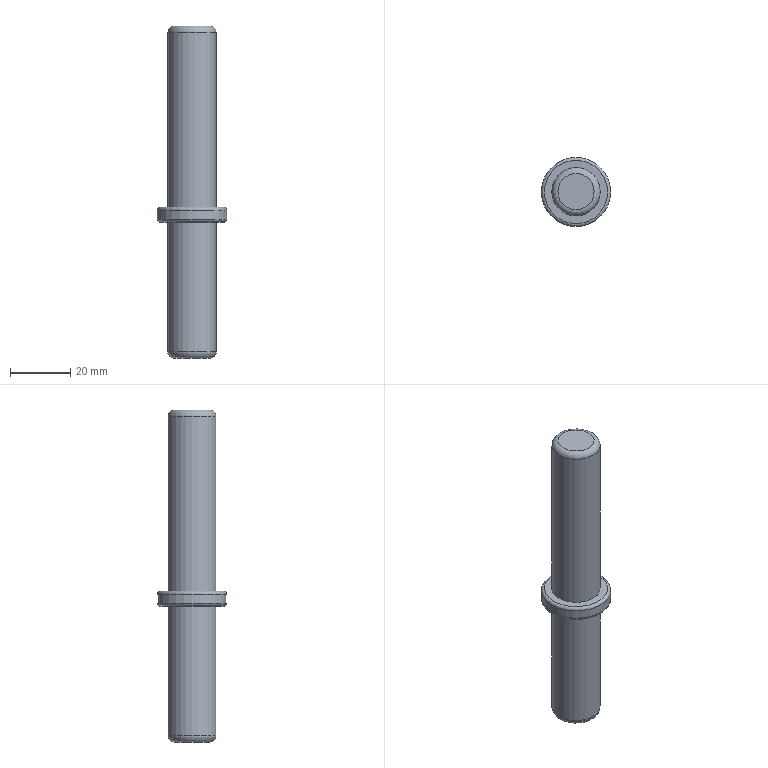Part | STEP file | 1 solid | 11 faces | box 23 x 23 x 110 mm | volume 23077 mm3 | plane 4 | torus 4 | cylinder 3 | commonest cylinder face diameters 16 x2 23 x1
STEP:
#1=CARTESIAN_POINT('',(0.,0.,0.));
#2=DIRECTION('',(0.,0.,1.));
#3=DIRECTION('',(1.,0.,0.));
#4=AXIS2_PLACEMENT_3D('',#1,#2,#3);
#5=CARTESIAN_POINT('',(1348.247,516.48,21.819));
#6=VERTEX_POINT('',#5);
#7=CARTESIAN_POINT('',(1340.247,516.48,21.819));
#8=DIRECTION('',(0.,0.,-1.));
#9=DIRECTION('',(1.,0.,0.));
#10=AXIS2_PLACEMENT_3D('',#7,#8,#9);
#11=CIRCLE('',#10,8.);
#12=CARTESIAN_POINT('',(1340.247,516.48,-41.181));
#13=DIRECTION('',(0.,0.,1.));
#14=DIRECTION('',(-1.,0.,0.));
#15=AXIS2_PLACEMENT_3D('',#12,#13,#14);
#16=CYLINDRICAL_SURFACE('',#15,8.);
#17=CARTESIAN_POINT('',(9.425,63.));
#18=DIRECTION('',(-1.,0.));
#19=VECTOR('',#18,1.);
#20=LINE('',#17,#19);
#21=(GEOMETRIC_REPRESENTATION_CONTEXT(2)PARAMETRIC_REPRESENTATION_CONTEXT()REPRESENTATION_CONTEXT('',''));
#22=DEFINITIONAL_REPRESENTATION('',(#20),#21);
#23=PCURVE('',#16,#22);
#24=CARTESIAN_POINT('',(1340.247,516.48,21.819));
#25=DIRECTION('',(0.,0.,1.));
#26=DIRECTION('',(-1.,0.,0.));
#27=AXIS2_PLACEMENT_3D('',#24,#25,#26);
#28=TOROIDAL_SURFACE('',#27,6.,2.);
#29=CARTESIAN_POINT('',(9.425,6.283));
#30=DIRECTION('',(-1.,0.));
#31=VECTOR('',#30,1.);
#32=LINE('',#29,#31);
#33=(GEOMETRIC_REPRESENTATION_CONTEXT(2)PARAMETRIC_REPRESENTATION_CONTEXT()REPRESENTATION_CONTEXT('',''));
#34=DEFINITIONAL_REPRESENTATION('',(#32),#33);
#35=PCURVE('',#28,#34);
#36=SURFACE_CURVE('',#11,(#23,#35),.PCURVE_S1.);
#37=EDGE_CURVE('',#6,#6,#36,.T.);
#38=ORIENTED_EDGE('',*,*,#37,.T.);
#39=CARTESIAN_POINT('',(1348.247,516.48,-36.181));
#40=VERTEX_POINT('',#39);
#41=CARTESIAN_POINT('',(1348.247,516.48,-36.181));
#42=CARTESIAN_POINT('',(1348.247,516.48,21.819));
#43=B_SPLINE_CURVE_WITH_KNOTS('',1,(#41,#42),.UNSPECIFIED.,.F.,.F.,(2,2),(5.,63.),.PIECEWISE_BEZIER_KNOTS.);
#44=CARTESIAN_POINT('',(3.142,0.));
#45=DIRECTION('',(0.,1.));
#46=VECTOR('',#45,1.);
#47=LINE('',#44,#46);
#48=(GEOMETRIC_REPRESENTATION_CONTEXT(2)PARAMETRIC_REPRESENTATION_CONTEXT()REPRESENTATION_CONTEXT('',''));
#49=DEFINITIONAL_REPRESENTATION('',(#47),#48);
#50=PCURVE('',#16,#49);
#51=CARTESIAN_POINT('',(9.425,0.));
#52=DIRECTION('',(0.,1.));
#53=VECTOR('',#52,1.);
#54=LINE('',#51,#53);
#55=(GEOMETRIC_REPRESENTATION_CONTEXT(2)PARAMETRIC_REPRESENTATION_CONTEXT()REPRESENTATION_CONTEXT('',''));
#56=DEFINITIONAL_REPRESENTATION('',(#54),#55);
#57=PCURVE('',#16,#56);
#58=SEAM_CURVE('',#43,(#50,#57),.PCURVE_S1.);
#59=EDGE_CURVE('',#40,#6,#58,.T.);
#60=ORIENTED_EDGE('',*,*,#59,.F.);
#61=CARTESIAN_POINT('',(1340.247,516.48,-36.181));
#62=DIRECTION('',(0.,0.,-1.));
#63=DIRECTION('',(1.,0.,0.));
#64=AXIS2_PLACEMENT_3D('',#61,#62,#63);
#65=CIRCLE('',#64,8.);
#66=CARTESIAN_POINT('',(9.425,5.));
#67=DIRECTION('',(-1.,0.));
#68=VECTOR('',#67,1.);
#69=LINE('',#66,#68);
#70=(GEOMETRIC_REPRESENTATION_CONTEXT(2)PARAMETRIC_REPRESENTATION_CONTEXT()REPRESENTATION_CONTEXT('',''));
#71=DEFINITIONAL_REPRESENTATION('',(#69),#70);
#72=PCURVE('',#16,#71);
#73=CARTESIAN_POINT('',(1340.247,516.48,-36.181));
#74=DIRECTION('',(0.,0.,1.));
#75=DIRECTION('',(-1.,0.,0.));
#76=AXIS2_PLACEMENT_3D('',#73,#74,#75);
#77=PLANE('',#76);
#78=CARTESIAN_POINT('',(-8.,0.));
#79=CARTESIAN_POINT('',(-8.,13.856));
#80=CARTESIAN_POINT('',(4.,6.928));
#81=CARTESIAN_POINT('',(16.,0.));
#82=CARTESIAN_POINT('',(4.,-6.928));
#83=CARTESIAN_POINT('',(-8.,-13.856));
#84=CARTESIAN_POINT('',(-8.,0.));
#85=(BOUNDED_CURVE()B_SPLINE_CURVE(2,(#78,#79,#80,#81,#82,#83,#84),.UNSPECIFIED.,.T.,.F.)B_SPLINE_CURVE_WITH_KNOTS((1,2,2,2,2,1),(-2.094,0.,2.094,4.189,6.283,8.378),.UNSPECIFIED.)CURVE()GEOMETRIC_REPRESENTATION_ITEM()RATIONAL_B_SPLINE_CURVE((1.,0.5,1.,0.5,1.,0.5,1.))REPRESENTATION_ITEM(''));
#86=(GEOMETRIC_REPRESENTATION_CONTEXT(2)PARAMETRIC_REPRESENTATION_CONTEXT()REPRESENTATION_CONTEXT('',''));
#87=DEFINITIONAL_REPRESENTATION('',(#85),#86);
#88=PCURVE('',#77,#87);
#89=SURFACE_CURVE('',#65,(#72,#88),.PCURVE_S1.);
#90=EDGE_CURVE('',#40,#40,#89,.T.);
#91=ORIENTED_EDGE('',*,*,#90,.F.);
#92=ORIENTED_EDGE('',*,*,#59,.T.);
#93=EDGE_LOOP('',(#38,#60,#91,#92));
#94=FACE_BOUND('',#93,.T.);
#95=ADVANCED_FACE('',(#94),#16,.T.);
#96=CARTESIAN_POINT('',(1351.747,516.48,-37.181));
#97=VERTEX_POINT('',#96);
#98=CARTESIAN_POINT('',(1340.247,516.48,-37.181));
#99=DIRECTION('',(0.,0.,-1.));
#100=DIRECTION('',(1.,0.,0.));
#101=AXIS2_PLACEMENT_3D('',#98,#99,#100);
#102=CIRCLE('',#101,11.5);
#103=CARTESIAN_POINT('',(1340.247,516.48,-41.181));
#104=DIRECTION('',(0.,0.,1.));
#105=DIRECTION('',(-1.,0.,0.));
#106=AXIS2_PLACEMENT_3D('',#103,#104,#105);
#107=CYLINDRICAL_SURFACE('',#106,11.5);
#108=CARTESIAN_POINT('',(9.425,4.));
#109=DIRECTION('',(-1.,0.));
#110=VECTOR('',#109,1.);
#111=LINE('',#108,#110);
#112=(GEOMETRIC_REPRESENTATION_CONTEXT(2)PARAMETRIC_REPRESENTATION_CONTEXT()REPRESENTATION_CONTEXT('',''));
#113=DEFINITIONAL_REPRESENTATION('',(#111),#112);
#114=PCURVE('',#107,#113);
#115=CARTESIAN_POINT('',(1340.247,516.48,-37.181));
#116=DIRECTION('',(0.,0.,1.));
#117=DIRECTION('',(-1.,0.,0.));
#118=AXIS2_PLACEMENT_3D('',#115,#116,#117);
#119=TOROIDAL_SURFACE('',#118,10.5,1.);
#120=CARTESIAN_POINT('',(9.425,6.283));
#121=DIRECTION('',(-1.,0.));
#122=VECTOR('',#121,1.);
#123=LINE('',#120,#122);
#124=(GEOMETRIC_REPRESENTATION_CONTEXT(2)PARAMETRIC_REPRESENTATION_CONTEXT()REPRESENTATION_CONTEXT('',''));
#125=DEFINITIONAL_REPRESENTATION('',(#123),#124);
#126=PCURVE('',#119,#125);
#127=SURFACE_CURVE('',#102,(#114,#126),.PCURVE_S1.);
#128=EDGE_CURVE('',#97,#97,#127,.T.);
#129=ORIENTED_EDGE('',*,*,#128,.T.);
#130=CARTESIAN_POINT('',(1351.747,516.48,-40.181));
#131=VERTEX_POINT('',#130);
#132=CARTESIAN_POINT('',(1351.747,516.48,-40.181));
#133=CARTESIAN_POINT('',(1351.747,516.48,-37.181));
#134=B_SPLINE_CURVE_WITH_KNOTS('',1,(#132,#133),.UNSPECIFIED.,.F.,.F.,(2,2),(1.,4.),.PIECEWISE_BEZIER_KNOTS.);
#135=CARTESIAN_POINT('',(3.142,0.));
#136=DIRECTION('',(0.,1.));
#137=VECTOR('',#136,1.);
#138=LINE('',#135,#137);
#139=(GEOMETRIC_REPRESENTATION_CONTEXT(2)PARAMETRIC_REPRESENTATION_CONTEXT()REPRESENTATION_CONTEXT('',''));
#140=DEFINITIONAL_REPRESENTATION('',(#138),#139);
#141=PCURVE('',#107,#140);
#142=CARTESIAN_POINT('',(9.425,0.));
#143=DIRECTION('',(0.,1.));
#144=VECTOR('',#143,1.);
#145=LINE('',#142,#144);
#146=(GEOMETRIC_REPRESENTATION_CONTEXT(2)PARAMETRIC_REPRESENTATION_CONTEXT()REPRESENTATION_CONTEXT('',''));
#147=DEFINITIONAL_REPRESENTATION('',(#145),#146);
#148=PCURVE('',#107,#147);
#149=SEAM_CURVE('',#134,(#141,#148),.PCURVE_S1.);
#150=EDGE_CURVE('',#131,#97,#149,.T.);
#151=ORIENTED_EDGE('',*,*,#150,.F.);
#152=CARTESIAN_POINT('',(1340.247,516.48,-40.181));
#153=DIRECTION('',(0.,0.,1.));
#154=DIRECTION('',(1.,0.,0.));
#155=AXIS2_PLACEMENT_3D('',#152,#153,#154);
#156=CIRCLE('',#155,11.5);
#157=CARTESIAN_POINT('',(3.142,1.));
#158=DIRECTION('',(1.,0.));
#159=VECTOR('',#158,1.);
#160=LINE('',#157,#159);
#161=(GEOMETRIC_REPRESENTATION_CONTEXT(2)PARAMETRIC_REPRESENTATION_CONTEXT()REPRESENTATION_CONTEXT('',''));
#162=DEFINITIONAL_REPRESENTATION('',(#160),#161);
#163=PCURVE('',#107,#162);
#164=CARTESIAN_POINT('',(1340.247,516.48,-40.181));
#165=DIRECTION('',(0.,0.,1.));
#166=DIRECTION('',(-1.,0.,0.));
#167=AXIS2_PLACEMENT_3D('',#164,#165,#166);
#168=TOROIDAL_SURFACE('',#167,10.5,1.);
#169=CARTESIAN_POINT('',(3.142,6.283));
#170=DIRECTION('',(1.,0.));
#171=VECTOR('',#170,1.);
#172=LINE('',#169,#171);
#173=(GEOMETRIC_REPRESENTATION_CONTEXT(2)PARAMETRIC_REPRESENTATION_CONTEXT()REPRESENTATION_CONTEXT('',''));
#174=DEFINITIONAL_REPRESENTATION('',(#172),#173);
#175=PCURVE('',#168,#174);
#176=SURFACE_CURVE('',#156,(#163,#175),.PCURVE_S1.);
#177=EDGE_CURVE('',#131,#131,#176,.T.);
#178=ORIENTED_EDGE('',*,*,#177,.T.);
#179=ORIENTED_EDGE('',*,*,#150,.T.);
#180=EDGE_LOOP('',(#129,#151,#178,#179));
#181=FACE_BOUND('',#180,.T.);
#182=ADVANCED_FACE('',(#181),#107,.T.);
#183=CARTESIAN_POINT('',(1350.747,516.48,-36.181));
#184=VERTEX_POINT('',#183);
#185=CARTESIAN_POINT('',(1340.247,516.48,-36.181));
#186=DIRECTION('',(0.,0.,1.));
#187=DIRECTION('',(1.,0.,0.));
#188=AXIS2_PLACEMENT_3D('',#185,#186,#187);
#189=CIRCLE('',#188,10.5);
#190=CARTESIAN_POINT('',(0.,0.));
#191=DIRECTION('',(-1.,0.));
#192=AXIS2_PLACEMENT_2D('',#190,#191);
#193=CIRCLE('',#192,10.5);
#194=(GEOMETRIC_REPRESENTATION_CONTEXT(2)PARAMETRIC_REPRESENTATION_CONTEXT()REPRESENTATION_CONTEXT('',''));
#195=DEFINITIONAL_REPRESENTATION('',(#193),#194);
#196=PCURVE('',#77,#195);
#197=CARTESIAN_POINT('',(3.142,7.854));
#198=DIRECTION('',(1.,0.));
#199=VECTOR('',#198,1.);
#200=LINE('',#197,#199);
#201=(GEOMETRIC_REPRESENTATION_CONTEXT(2)PARAMETRIC_REPRESENTATION_CONTEXT()REPRESENTATION_CONTEXT('',''));
#202=DEFINITIONAL_REPRESENTATION('',(#200),#201);
#203=PCURVE('',#119,#202);
#204=SURFACE_CURVE('',#189,(#196,#203),.PCURVE_S1.);
#205=EDGE_CURVE('',#184,#184,#204,.T.);
#206=ORIENTED_EDGE('',*,*,#205,.T.);
#207=EDGE_LOOP('',(#206));
#208=FACE_BOUND('',#207,.T.);
#209=ORIENTED_EDGE('',*,*,#90,.T.);
#210=EDGE_LOOP('',(#209));
#211=FACE_BOUND('',#210,.T.);
#212=ADVANCED_FACE('',(#208,#211),#77,.T.);
#213=CARTESIAN_POINT('',(1350.747,516.48,-41.181));
#214=VERTEX_POINT('',#213);
#215=CARTESIAN_POINT('',(1340.247,516.48,-41.181));
#216=DIRECTION('',(0.,0.,-1.));
#217=DIRECTION('',(1.,0.,0.));
#218=AXIS2_PLACEMENT_3D('',#215,#216,#217);
#219=CIRCLE('',#218,10.5);
#220=CARTESIAN_POINT('',(1340.247,516.48,-41.181));
#221=DIRECTION('',(0.,0.,1.));
#222=DIRECTION('',(-1.,0.,0.));
#223=AXIS2_PLACEMENT_3D('',#220,#221,#222);
#224=PLANE('',#223);
#225=CARTESIAN_POINT('',(-10.5,0.));
#226=CARTESIAN_POINT('',(-10.5,18.187));
#227=CARTESIAN_POINT('',(5.25,9.093));
#228=CARTESIAN_POINT('',(21.,0.));
#229=CARTESIAN_POINT('',(5.25,-9.093));
#230=CARTESIAN_POINT('',(-10.5,-18.187));
#231=CARTESIAN_POINT('',(-10.5,0.));
#232=(BOUNDED_CURVE()B_SPLINE_CURVE(2,(#225,#226,#227,#228,#229,#230,#231),.UNSPECIFIED.,.T.,.F.)B_SPLINE_CURVE_WITH_KNOTS((1,2,2,2,2,1),(-2.094,0.,2.094,4.189,6.283,8.378),.UNSPECIFIED.)CURVE()GEOMETRIC_REPRESENTATION_ITEM()RATIONAL_B_SPLINE_CURVE((1.,0.5,1.,0.5,1.,0.5,1.))REPRESENTATION_ITEM(''));
#233=(GEOMETRIC_REPRESENTATION_CONTEXT(2)PARAMETRIC_REPRESENTATION_CONTEXT()REPRESENTATION_CONTEXT('',''));
#234=DEFINITIONAL_REPRESENTATION('',(#232),#233);
#235=PCURVE('',#224,#234);
#236=CARTESIAN_POINT('',(9.425,4.712));
#237=DIRECTION('',(-1.,0.));
#238=VECTOR('',#237,1.);
#239=LINE('',#236,#238);
#240=(GEOMETRIC_REPRESENTATION_CONTEXT(2)PARAMETRIC_REPRESENTATION_CONTEXT()REPRESENTATION_CONTEXT('',''));
#241=DEFINITIONAL_REPRESENTATION('',(#239),#240);
#242=PCURVE('',#168,#241);
#243=SURFACE_CURVE('',#219,(#235,#242),.PCURVE_S1.);
#244=EDGE_CURVE('',#214,#214,#243,.T.);
#245=ORIENTED_EDGE('',*,*,#244,.T.);
#246=EDGE_LOOP('',(#245));
#247=FACE_BOUND('',#246,.T.);
#248=CARTESIAN_POINT('',(1348.247,516.48,-41.181));
#249=VERTEX_POINT('',#248);
#250=CARTESIAN_POINT('',(1340.247,516.48,-41.181));
#251=DIRECTION('',(0.,0.,1.));
#252=DIRECTION('',(1.,0.,0.));
#253=AXIS2_PLACEMENT_3D('',#250,#251,#252);
#254=CIRCLE('',#253,8.);
#255=CARTESIAN_POINT('',(0.,0.));
#256=DIRECTION('',(-1.,0.));
#257=AXIS2_PLACEMENT_2D('',#255,#256);
#258=CIRCLE('',#257,8.);
#259=(GEOMETRIC_REPRESENTATION_CONTEXT(2)PARAMETRIC_REPRESENTATION_CONTEXT()REPRESENTATION_CONTEXT('',''));
#260=DEFINITIONAL_REPRESENTATION('',(#258),#259);
#261=PCURVE('',#224,#260);
#262=CARTESIAN_POINT('',(1340.247,516.48,-41.181));
#263=DIRECTION('',(0.,0.,-1.));
#264=DIRECTION('',(1.,0.,0.));
#265=AXIS2_PLACEMENT_3D('',#262,#263,#264);
#266=CYLINDRICAL_SURFACE('',#265,8.);
#267=CARTESIAN_POINT('',(6.283,0.));
#268=DIRECTION('',(-1.,0.));
#269=VECTOR('',#268,1.);
#270=LINE('',#267,#269);
#271=(GEOMETRIC_REPRESENTATION_CONTEXT(2)PARAMETRIC_REPRESENTATION_CONTEXT()REPRESENTATION_CONTEXT('',''));
#272=DEFINITIONAL_REPRESENTATION('',(#270),#271);
#273=PCURVE('',#266,#272);
#274=SURFACE_CURVE('',#254,(#261,#273),.PCURVE_S1.);
#275=EDGE_CURVE('',#249,#249,#274,.T.);
#276=ORIENTED_EDGE('',*,*,#275,.T.);
#277=EDGE_LOOP('',(#276));
#278=FACE_BOUND('',#277,.T.);
#279=ADVANCED_FACE('',(#247,#278),#224,.F.);
#280=CARTESIAN_POINT('',(1348.247,516.48,-84.181));
#281=VERTEX_POINT('',#280);
#282=CARTESIAN_POINT('',(1340.247,516.48,-84.181));
#283=DIRECTION('',(0.,0.,1.));
#284=DIRECTION('',(1.,0.,0.));
#285=AXIS2_PLACEMENT_3D('',#282,#283,#284);
#286=CIRCLE('',#285,8.);
#287=CARTESIAN_POINT('',(6.283,43.));
#288=DIRECTION('',(-1.,0.));
#289=VECTOR('',#288,1.);
#290=LINE('',#287,#289);
#291=(GEOMETRIC_REPRESENTATION_CONTEXT(2)PARAMETRIC_REPRESENTATION_CONTEXT()REPRESENTATION_CONTEXT('',''));
#292=DEFINITIONAL_REPRESENTATION('',(#290),#291);
#293=PCURVE('',#266,#292);
#294=CARTESIAN_POINT('',(1340.247,516.48,-84.181));
#295=DIRECTION('',(0.,0.,1.));
#296=DIRECTION('',(-1.,0.,0.));
#297=AXIS2_PLACEMENT_3D('',#294,#295,#296);
#298=TOROIDAL_SURFACE('',#297,6.,2.);
#299=CARTESIAN_POINT('',(3.142,6.283));
#300=DIRECTION('',(1.,0.));
#301=VECTOR('',#300,1.);
#302=LINE('',#299,#301);
#303=(GEOMETRIC_REPRESENTATION_CONTEXT(2)PARAMETRIC_REPRESENTATION_CONTEXT()REPRESENTATION_CONTEXT('',''));
#304=DEFINITIONAL_REPRESENTATION('',(#302),#303);
#305=PCURVE('',#298,#304);
#306=SURFACE_CURVE('',#286,(#293,#305),.PCURVE_S1.);
#307=EDGE_CURVE('',#281,#281,#306,.T.);
#308=ORIENTED_EDGE('',*,*,#307,.T.);
#309=CARTESIAN_POINT('',(1348.247,516.48,-41.181));
#310=CARTESIAN_POINT('',(1348.247,516.48,-84.181));
#311=B_SPLINE_CURVE_WITH_KNOTS('',1,(#309,#310),.UNSPECIFIED.,.F.,.F.,(2,2),(0.,43.),.PIECEWISE_BEZIER_KNOTS.);
#312=CARTESIAN_POINT('',(0.,0.));
#313=DIRECTION('',(0.,1.));
#314=VECTOR('',#313,1.);
#315=LINE('',#312,#314);
#316=(GEOMETRIC_REPRESENTATION_CONTEXT(2)PARAMETRIC_REPRESENTATION_CONTEXT()REPRESENTATION_CONTEXT('',''));
#317=DEFINITIONAL_REPRESENTATION('',(#315),#316);
#318=PCURVE('',#266,#317);
#319=CARTESIAN_POINT('',(6.283,0.));
#320=DIRECTION('',(0.,1.));
#321=VECTOR('',#320,1.);
#322=LINE('',#319,#321);
#323=(GEOMETRIC_REPRESENTATION_CONTEXT(2)PARAMETRIC_REPRESENTATION_CONTEXT()REPRESENTATION_CONTEXT('',''));
#324=DEFINITIONAL_REPRESENTATION('',(#322),#323);
#325=PCURVE('',#266,#324);
#326=SEAM_CURVE('',#311,(#318,#325),.PCURVE_S1.);
#327=EDGE_CURVE('',#249,#281,#326,.T.);
#328=ORIENTED_EDGE('',*,*,#327,.F.);
#329=ORIENTED_EDGE('',*,*,#275,.F.);
#330=ORIENTED_EDGE('',*,*,#327,.T.);
#331=EDGE_LOOP('',(#308,#328,#329,#330));
#332=FACE_BOUND('',#331,.T.);
#333=ADVANCED_FACE('',(#332),#266,.T.);
#334=ORIENTED_EDGE('',*,*,#128,.F.);
#335=CARTESIAN_POINT('',(1351.747,516.48,-37.181));
#336=CARTESIAN_POINT('',(1351.747,516.48,-36.914));
#337=CARTESIAN_POINT('',(1351.662,516.48,-36.653));
#338=CARTESIAN_POINT('',(1351.499,516.48,-36.429));
#339=CARTESIAN_POINT('',(1351.275,516.48,-36.266));
#340=CARTESIAN_POINT('',(1351.015,516.48,-36.181));
#341=CARTESIAN_POINT('',(1350.747,516.48,-36.181));
#342=(BOUNDED_CURVE()B_SPLINE_CURVE(6,(#335,#336,#337,#338,#339,#340,#341),.UNSPECIFIED.,.F.,.F.)B_SPLINE_CURVE_WITH_KNOTS((7,7),(0.,1.571),.PIECEWISE_BEZIER_KNOTS.)CURVE()GEOMETRIC_REPRESENTATION_ITEM()RATIONAL_B_SPLINE_CURVE((1.031,1.01,0.9979,0.994,0.9979,1.01,1.031))REPRESENTATION_ITEM(''));
#343=CARTESIAN_POINT('',(9.425,6.283));
#344=DIRECTION('',(0.,1.));
#345=VECTOR('',#344,1.);
#346=LINE('',#343,#345);
#347=(GEOMETRIC_REPRESENTATION_CONTEXT(2)PARAMETRIC_REPRESENTATION_CONTEXT()REPRESENTATION_CONTEXT('',''));
#348=DEFINITIONAL_REPRESENTATION('',(#346),#347);
#349=PCURVE('',#119,#348);
#350=CARTESIAN_POINT('',(3.142,6.283));
#351=DIRECTION('',(0.,1.));
#352=VECTOR('',#351,1.);
#353=LINE('',#350,#352);
#354=(GEOMETRIC_REPRESENTATION_CONTEXT(2)PARAMETRIC_REPRESENTATION_CONTEXT()REPRESENTATION_CONTEXT('',''));
#355=DEFINITIONAL_REPRESENTATION('',(#353),#354);
#356=PCURVE('',#119,#355);
#357=SEAM_CURVE('',#342,(#349,#356),.PCURVE_S1.);
#358=EDGE_CURVE('',#97,#184,#357,.T.);
#359=ORIENTED_EDGE('',*,*,#358,.T.);
#360=ORIENTED_EDGE('',*,*,#205,.F.);
#361=ORIENTED_EDGE('',*,*,#358,.F.);
#362=EDGE_LOOP('',(#334,#359,#360,#361));
#363=FACE_BOUND('',#362,.T.);
#364=ADVANCED_FACE('',(#363),#119,.T.);
#365=ORIENTED_EDGE('',*,*,#244,.F.);
#366=CARTESIAN_POINT('',(1350.747,516.48,-41.181));
#367=CARTESIAN_POINT('',(1351.015,516.48,-41.181));
#368=CARTESIAN_POINT('',(1351.275,516.48,-41.096));
#369=CARTESIAN_POINT('',(1351.499,516.48,-40.933));
#370=CARTESIAN_POINT('',(1351.662,516.48,-40.709));
#371=CARTESIAN_POINT('',(1351.747,516.48,-40.448));
#372=CARTESIAN_POINT('',(1351.747,516.48,-40.181));
#373=(BOUNDED_CURVE()B_SPLINE_CURVE(6,(#366,#367,#368,#369,#370,#371,#372),.UNSPECIFIED.,.F.,.F.)B_SPLINE_CURVE_WITH_KNOTS((7,7),(4.712,6.283),.PIECEWISE_BEZIER_KNOTS.)CURVE()GEOMETRIC_REPRESENTATION_ITEM()RATIONAL_B_SPLINE_CURVE((1.031,1.01,0.9979,0.994,0.9979,1.01,1.031))REPRESENTATION_ITEM(''));
#374=CARTESIAN_POINT('',(9.425,0.));
#375=DIRECTION('',(0.,1.));
#376=VECTOR('',#375,1.);
#377=LINE('',#374,#376);
#378=(GEOMETRIC_REPRESENTATION_CONTEXT(2)PARAMETRIC_REPRESENTATION_CONTEXT()REPRESENTATION_CONTEXT('',''));
#379=DEFINITIONAL_REPRESENTATION('',(#377),#378);
#380=PCURVE('',#168,#379);
#381=CARTESIAN_POINT('',(3.142,0.));
#382=DIRECTION('',(0.,1.));
#383=VECTOR('',#382,1.);
#384=LINE('',#381,#383);
#385=(GEOMETRIC_REPRESENTATION_CONTEXT(2)PARAMETRIC_REPRESENTATION_CONTEXT()REPRESENTATION_CONTEXT('',''));
#386=DEFINITIONAL_REPRESENTATION('',(#384),#385);
#387=PCURVE('',#168,#386);
#388=SEAM_CURVE('',#373,(#380,#387),.PCURVE_S1.);
#389=EDGE_CURVE('',#214,#131,#388,.T.);
#390=ORIENTED_EDGE('',*,*,#389,.T.);
#391=ORIENTED_EDGE('',*,*,#177,.F.);
#392=ORIENTED_EDGE('',*,*,#389,.F.);
#393=EDGE_LOOP('',(#365,#390,#391,#392));
#394=FACE_BOUND('',#393,.T.);
#395=ADVANCED_FACE('',(#394),#168,.T.);
#396=ORIENTED_EDGE('',*,*,#37,.F.);
#397=CARTESIAN_POINT('',(1346.247,516.48,23.819));
#398=VERTEX_POINT('',#397);
#399=CARTESIAN_POINT('',(1348.247,516.48,21.819));
#400=CARTESIAN_POINT('',(1348.247,516.48,22.354));
#401=CARTESIAN_POINT('',(1348.077,516.48,22.874));
#402=CARTESIAN_POINT('',(1347.751,516.48,23.323));
#403=CARTESIAN_POINT('',(1347.303,516.48,23.649));
#404=CARTESIAN_POINT('',(1346.782,516.48,23.819));
#405=CARTESIAN_POINT('',(1346.247,516.48,23.819));
#406=(BOUNDED_CURVE()B_SPLINE_CURVE(6,(#399,#400,#401,#402,#403,#404,#405),.UNSPECIFIED.,.F.,.F.)B_SPLINE_CURVE_WITH_KNOTS((7,7),(0.,1.571),.PIECEWISE_BEZIER_KNOTS.)CURVE()GEOMETRIC_REPRESENTATION_ITEM()RATIONAL_B_SPLINE_CURVE((1.031,1.01,0.9979,0.994,0.9979,1.01,1.031))REPRESENTATION_ITEM(''));
#407=CARTESIAN_POINT('',(9.425,6.283));
#408=DIRECTION('',(0.,1.));
#409=VECTOR('',#408,1.);
#410=LINE('',#407,#409);
#411=(GEOMETRIC_REPRESENTATION_CONTEXT(2)PARAMETRIC_REPRESENTATION_CONTEXT()REPRESENTATION_CONTEXT('',''));
#412=DEFINITIONAL_REPRESENTATION('',(#410),#411);
#413=PCURVE('',#28,#412);
#414=CARTESIAN_POINT('',(3.142,6.283));
#415=DIRECTION('',(0.,1.));
#416=VECTOR('',#415,1.);
#417=LINE('',#414,#416);
#418=(GEOMETRIC_REPRESENTATION_CONTEXT(2)PARAMETRIC_REPRESENTATION_CONTEXT()REPRESENTATION_CONTEXT('',''));
#419=DEFINITIONAL_REPRESENTATION('',(#417),#418);
#420=PCURVE('',#28,#419);
#421=SEAM_CURVE('',#406,(#413,#420),.PCURVE_S1.);
#422=EDGE_CURVE('',#6,#398,#421,.T.);
#423=ORIENTED_EDGE('',*,*,#422,.T.);
#424=CARTESIAN_POINT('',(1340.247,516.48,23.819));
#425=DIRECTION('',(0.,0.,1.));
#426=DIRECTION('',(1.,0.,0.));
#427=AXIS2_PLACEMENT_3D('',#424,#425,#426);
#428=CIRCLE('',#427,6.);
#429=CARTESIAN_POINT('',(3.142,7.854));
#430=DIRECTION('',(1.,0.));
#431=VECTOR('',#430,1.);
#432=LINE('',#429,#431);
#433=(GEOMETRIC_REPRESENTATION_CONTEXT(2)PARAMETRIC_REPRESENTATION_CONTEXT()REPRESENTATION_CONTEXT('',''));
#434=DEFINITIONAL_REPRESENTATION('',(#432),#433);
#435=PCURVE('',#28,#434);
#436=CARTESIAN_POINT('',(1534.247,516.48,23.819));
#437=DIRECTION('',(0.,0.,1.));
#438=DIRECTION('',(1.,0.,0.));
#439=AXIS2_PLACEMENT_3D('',#436,#437,#438);
#440=PLANE('',#439);
#441=CARTESIAN_POINT('',(-194.,0.));
#442=DIRECTION('',(1.,0.));
#443=AXIS2_PLACEMENT_2D('',#441,#442);
#444=CIRCLE('',#443,6.);
#445=(GEOMETRIC_REPRESENTATION_CONTEXT(2)PARAMETRIC_REPRESENTATION_CONTEXT()REPRESENTATION_CONTEXT('',''));
#446=DEFINITIONAL_REPRESENTATION('',(#444),#445);
#447=PCURVE('',#440,#446);
#448=SURFACE_CURVE('',#428,(#435,#447),.PCURVE_S1.);
#449=EDGE_CURVE('',#398,#398,#448,.T.);
#450=ORIENTED_EDGE('',*,*,#449,.F.);
#451=ORIENTED_EDGE('',*,*,#422,.F.);
#452=EDGE_LOOP('',(#396,#423,#450,#451));
#453=FACE_BOUND('',#452,.T.);
#454=ADVANCED_FACE('',(#453),#28,.T.);
#455=CARTESIAN_POINT('',(1346.247,516.48,-86.181));
#456=VERTEX_POINT('',#455);
#457=CARTESIAN_POINT('',(1340.247,516.48,-86.181));
#458=DIRECTION('',(0.,0.,-1.));
#459=DIRECTION('',(1.,0.,0.));
#460=AXIS2_PLACEMENT_3D('',#457,#458,#459);
#461=CIRCLE('',#460,6.);
#462=CARTESIAN_POINT('',(9.425,4.712));
#463=DIRECTION('',(-1.,0.));
#464=VECTOR('',#463,1.);
#465=LINE('',#462,#464);
#466=(GEOMETRIC_REPRESENTATION_CONTEXT(2)PARAMETRIC_REPRESENTATION_CONTEXT()REPRESENTATION_CONTEXT('',''));
#467=DEFINITIONAL_REPRESENTATION('',(#465),#466);
#468=PCURVE('',#298,#467);
#469=CARTESIAN_POINT('',(1534.247,516.48,-86.181));
#470=DIRECTION('',(0.,0.,1.));
#471=DIRECTION('',(1.,0.,0.));
#472=AXIS2_PLACEMENT_3D('',#469,#470,#471);
#473=PLANE('',#472);
#474=CARTESIAN_POINT('',(-188.,0.));
#475=CARTESIAN_POINT('',(-188.,-10.392));
#476=CARTESIAN_POINT('',(-197.,-5.196));
#477=CARTESIAN_POINT('',(-206.,0.));
#478=CARTESIAN_POINT('',(-197.,5.196));
#479=CARTESIAN_POINT('',(-188.,10.392));
#480=CARTESIAN_POINT('',(-188.,0.));
#481=(BOUNDED_CURVE()B_SPLINE_CURVE(2,(#474,#475,#476,#477,#478,#479,#480),.UNSPECIFIED.,.T.,.F.)B_SPLINE_CURVE_WITH_KNOTS((1,2,2,2,2,1),(-2.094,0.,2.094,4.189,6.283,8.378),.UNSPECIFIED.)CURVE()GEOMETRIC_REPRESENTATION_ITEM()RATIONAL_B_SPLINE_CURVE((1.,0.5,1.,0.5,1.,0.5,1.))REPRESENTATION_ITEM(''));
#482=(GEOMETRIC_REPRESENTATION_CONTEXT(2)PARAMETRIC_REPRESENTATION_CONTEXT()REPRESENTATION_CONTEXT('',''));
#483=DEFINITIONAL_REPRESENTATION('',(#481),#482);
#484=PCURVE('',#473,#483);
#485=SURFACE_CURVE('',#461,(#468,#484),.PCURVE_S1.);
#486=EDGE_CURVE('',#456,#456,#485,.T.);
#487=ORIENTED_EDGE('',*,*,#486,.F.);
#488=CARTESIAN_POINT('',(1346.247,516.48,-86.181));
#489=CARTESIAN_POINT('',(1346.782,516.48,-86.181));
#490=CARTESIAN_POINT('',(1347.303,516.48,-86.011));
#491=CARTESIAN_POINT('',(1347.751,516.48,-85.685));
#492=CARTESIAN_POINT('',(1348.077,516.48,-85.236));
#493=CARTESIAN_POINT('',(1348.247,516.48,-84.716));
#494=CARTESIAN_POINT('',(1348.247,516.48,-84.181));
#495=(BOUNDED_CURVE()B_SPLINE_CURVE(6,(#488,#489,#490,#491,#492,#493,#494),.UNSPECIFIED.,.F.,.F.)B_SPLINE_CURVE_WITH_KNOTS((7,7),(4.712,6.283),.PIECEWISE_BEZIER_KNOTS.)CURVE()GEOMETRIC_REPRESENTATION_ITEM()RATIONAL_B_SPLINE_CURVE((1.031,1.01,0.9979,0.994,0.9979,1.01,1.031))REPRESENTATION_ITEM(''));
#496=CARTESIAN_POINT('',(9.425,0.));
#497=DIRECTION('',(0.,1.));
#498=VECTOR('',#497,1.);
#499=LINE('',#496,#498);
#500=(GEOMETRIC_REPRESENTATION_CONTEXT(2)PARAMETRIC_REPRESENTATION_CONTEXT()REPRESENTATION_CONTEXT('',''));
#501=DEFINITIONAL_REPRESENTATION('',(#499),#500);
#502=PCURVE('',#298,#501);
#503=CARTESIAN_POINT('',(3.142,0.));
#504=DIRECTION('',(0.,1.));
#505=VECTOR('',#504,1.);
#506=LINE('',#503,#505);
#507=(GEOMETRIC_REPRESENTATION_CONTEXT(2)PARAMETRIC_REPRESENTATION_CONTEXT()REPRESENTATION_CONTEXT('',''));
#508=DEFINITIONAL_REPRESENTATION('',(#506),#507);
#509=PCURVE('',#298,#508);
#510=SEAM_CURVE('',#495,(#502,#509),.PCURVE_S1.);
#511=EDGE_CURVE('',#456,#281,#510,.T.);
#512=ORIENTED_EDGE('',*,*,#511,.T.);
#513=ORIENTED_EDGE('',*,*,#307,.F.);
#514=ORIENTED_EDGE('',*,*,#511,.F.);
#515=EDGE_LOOP('',(#487,#512,#513,#514));
#516=FACE_BOUND('',#515,.T.);
#517=ADVANCED_FACE('',(#516),#298,.T.);
#518=ORIENTED_EDGE('',*,*,#486,.T.);
#519=EDGE_LOOP('',(#518));
#520=FACE_BOUND('',#519,.T.);
#521=ADVANCED_FACE('',(#520),#473,.F.);
#522=ORIENTED_EDGE('',*,*,#449,.T.);
#523=EDGE_LOOP('',(#522));
#524=FACE_BOUND('',#523,.T.);
#525=ADVANCED_FACE('',(#524),#440,.T.);
#526=CLOSED_SHELL('',(#95,#182,#212,#279,#333,#364,#395,#454,#517,#521,#525));
#527=MANIFOLD_SOLID_BREP('',#526);
#528=(LENGTH_UNIT()NAMED_UNIT(*)SI_UNIT(.MILLI.,.METRE.));
#529=UNCERTAINTY_MEASURE_WITH_UNIT(LENGTH_MEASURE(0.00001),#528,'','');
#530=(NAMED_UNIT(*)PLANE_ANGLE_UNIT()SI_UNIT($,.RADIAN.));
#531=(NAMED_UNIT(*)SI_UNIT($,.STERADIAN.)SOLID_ANGLE_UNIT());
#532=(GEOMETRIC_REPRESENTATION_CONTEXT(3)GLOBAL_UNCERTAINTY_ASSIGNED_CONTEXT((#529))GLOBAL_UNIT_ASSIGNED_CONTEXT((#528,#530,#531))REPRESENTATION_CONTEXT('',''));
#533=ADVANCED_BREP_SHAPE_REPRESENTATION('',(#4,#527),#532);